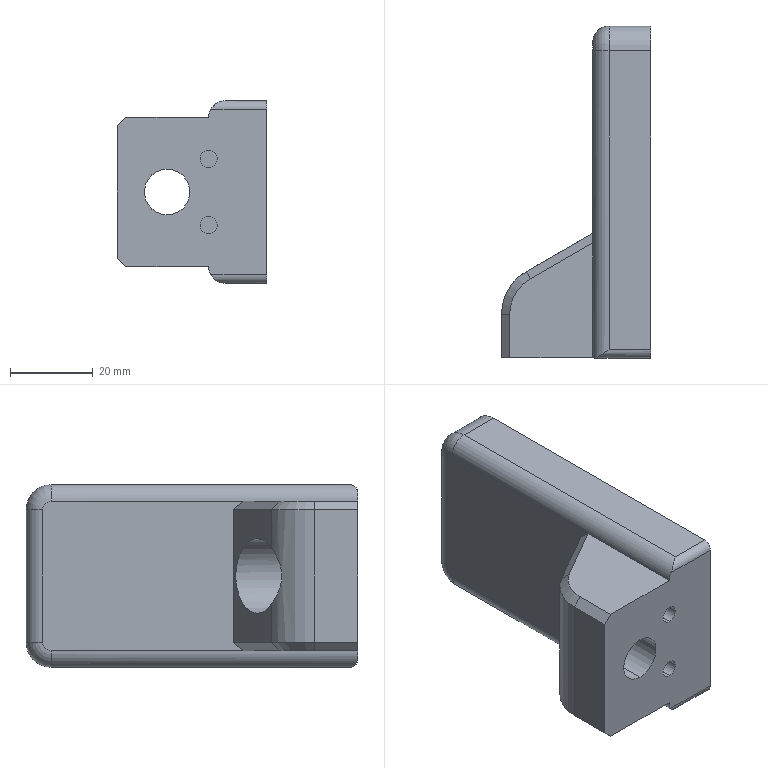Part | NX | features BREP 1 | 1 solid | 37 faces | box 36 x 80 x 44 mm | volume 61512 mm3 | plane 17 | cylinder 16 | cone 2 | torus 2 | commonest cylinder face diameters 4.1 x4 8 x3 4 x2 11 x2 12 x2 18 x2
STEP:
#1=CARTESIAN_POINT('',(-84.,294.703,-10.05));
#2=VERTEX_POINT('',#1);
#3=CARTESIAN_POINT('',(-84.,294.703,-5.95));
#4=VERTEX_POINT('',#3);
#5=CARTESIAN_POINT('',(-84.,294.703,-8.));
#6=DIRECTION('',(0.,-1.,0.));
#7=DIRECTION('',(0.,0.,1.));
#8=AXIS2_PLACEMENT_3D('',#5,#6,#7);
#9=CIRCLE('',#8,2.05);
#10=EDGE_CURVE('',#2,#4,#9,.T.);
#11=ORIENTED_EDGE('',*,*,#10,.F.);
#12=CARTESIAN_POINT('',(-84.,284.703,-10.05));
#13=VERTEX_POINT('',#12);
#14=CARTESIAN_POINT('',(-84.,294.703,-10.05));
#15=DIRECTION('',(0.,-1.,0.));
#16=VECTOR('',#15,1000.);
#17=LINE('',#14,#16);
#18=EDGE_CURVE('',#2,#13,#17,.T.);
#19=ORIENTED_EDGE('',*,*,#18,.T.);
#20=CARTESIAN_POINT('',(-84.,284.703,-5.95));
#21=VERTEX_POINT('',#20);
#22=CARTESIAN_POINT('',(-84.,284.703,-8.));
#23=DIRECTION('',(0.,-1.,0.));
#24=DIRECTION('',(0.,0.,1.));
#25=AXIS2_PLACEMENT_3D('',#22,#23,#24);
#26=CIRCLE('',#25,2.05);
#27=EDGE_CURVE('',#13,#21,#26,.T.);
#28=ORIENTED_EDGE('',*,*,#27,.T.);
#29=CARTESIAN_POINT('',(-84.,294.703,-5.95));
#30=DIRECTION('',(0.,1.,0.));
#31=VECTOR('',#30,1000.);
#32=LINE('',#29,#31);
#33=EDGE_CURVE('',#21,#4,#32,.T.);
#34=ORIENTED_EDGE('',*,*,#33,.T.);
#35=EDGE_LOOP('',(#11,#19,#28,#34));
#36=FACE_BOUND('',#35,.T.);
#37=CARTESIAN_POINT('',(-84.,294.703,-8.));
#38=DIRECTION('',(0.,-1.,0.));
#39=DIRECTION('',(0.,0.,-1.));
#40=AXIS2_PLACEMENT_3D('',#37,#38,#39);
#41=CYLINDRICAL_SURFACE('',#40,2.05);
#42=ADVANCED_FACE('',(#36),#41,.F.);
#43=CARTESIAN_POINT('',(-84.,294.703,5.95));
#44=VERTEX_POINT('',#43);
#45=CARTESIAN_POINT('',(-84.,294.703,10.05));
#46=VERTEX_POINT('',#45);
#47=CARTESIAN_POINT('',(-84.,294.703,8.));
#48=DIRECTION('',(0.,-1.,0.));
#49=DIRECTION('',(0.,0.,1.));
#50=AXIS2_PLACEMENT_3D('',#47,#48,#49);
#51=CIRCLE('',#50,2.05);
#52=EDGE_CURVE('',#44,#46,#51,.T.);
#53=ORIENTED_EDGE('',*,*,#52,.F.);
#54=CARTESIAN_POINT('',(-84.,284.703,5.95));
#55=VERTEX_POINT('',#54);
#56=CARTESIAN_POINT('',(-84.,294.703,5.95));
#57=DIRECTION('',(0.,1.,0.));
#58=VECTOR('',#57,1000.);
#59=LINE('',#56,#58);
#60=EDGE_CURVE('',#55,#44,#59,.T.);
#61=ORIENTED_EDGE('',*,*,#60,.F.);
#62=CARTESIAN_POINT('',(-84.,284.703,10.05));
#63=VERTEX_POINT('',#62);
#64=CARTESIAN_POINT('',(-84.,284.703,8.));
#65=DIRECTION('',(0.,-1.,0.));
#66=DIRECTION('',(0.,0.,1.));
#67=AXIS2_PLACEMENT_3D('',#64,#65,#66);
#68=CIRCLE('',#67,2.05);
#69=EDGE_CURVE('',#55,#63,#68,.T.);
#70=ORIENTED_EDGE('',*,*,#69,.T.);
#71=CARTESIAN_POINT('',(-84.,294.703,10.05));
#72=DIRECTION('',(0.,-1.,0.));
#73=VECTOR('',#72,1000.);
#74=LINE('',#71,#73);
#75=EDGE_CURVE('',#46,#63,#74,.T.);
#76=ORIENTED_EDGE('',*,*,#75,.F.);
#77=EDGE_LOOP('',(#53,#61,#70,#76));
#78=FACE_BOUND('',#77,.T.);
#79=CARTESIAN_POINT('',(-84.,294.703,8.));
#80=DIRECTION('',(0.,-1.,0.));
#81=DIRECTION('',(0.,0.,-1.));
#82=AXIS2_PLACEMENT_3D('',#79,#80,#81);
#83=CYLINDRICAL_SURFACE('',#82,2.05);
#84=ADVANCED_FACE('',(#78),#83,.F.);
#85=CARTESIAN_POINT('',(-94.,292.703,-9.));
#86=VERTEX_POINT('',#85);
#87=CARTESIAN_POINT('',(-94.,292.703,9.));
#88=VERTEX_POINT('',#87);
#89=CARTESIAN_POINT('',(-94.,292.703,0.));
#90=DIRECTION('',(0.,-1.,0.));
#91=DIRECTION('',(0.,0.,-1.));
#92=AXIS2_PLACEMENT_3D('',#89,#90,#91);
#93=CIRCLE('',#92,9.);
#94=EDGE_CURVE('',#86,#88,#93,.T.);
#95=ORIENTED_EDGE('',*,*,#94,.T.);
#96=CARTESIAN_POINT('',(-94.,308.93,9.));
#97=VERTEX_POINT('',#96);
#98=CARTESIAN_POINT('',(-94.,259.248,9.));
#99=DIRECTION('',(0.,-1.,0.));
#100=VECTOR('',#99,1000.);
#101=LINE('',#98,#100);
#102=EDGE_CURVE('',#97,#88,#101,.T.);
#103=ORIENTED_EDGE('',*,*,#102,.F.);
#104=CARTESIAN_POINT('',(-94.,308.93,-9.));
#105=VERTEX_POINT('',#104);
#106=CARTESIAN_POINT('',(-94.,308.93,-9.));
#107=CARTESIAN_POINT('',(-76.,319.322,-9.));
#108=CARTESIAN_POINT('',(-76.,319.322,9.));
#109=CARTESIAN_POINT('',(-94.,308.93,9.));
#110=(BOUNDED_CURVE()B_SPLINE_CURVE(3,(#106,#107,#108,#109),.UNSPECIFIED.,.F.,.F.)B_SPLINE_CURVE_WITH_KNOTS((4,4),(0.,1.),.PIECEWISE_BEZIER_KNOTS.)CURVE()GEOMETRIC_REPRESENTATION_ITEM()RATIONAL_B_SPLINE_CURVE((1.,0.3333,0.3333,1.))REPRESENTATION_ITEM(''));
#111=EDGE_CURVE('',#105,#97,#110,.T.);
#112=ORIENTED_EDGE('',*,*,#111,.F.);
#113=CARTESIAN_POINT('',(-94.,259.248,-9.));
#114=DIRECTION('',(0.,1.,0.));
#115=VECTOR('',#114,1000.);
#116=LINE('',#113,#115);
#117=EDGE_CURVE('',#86,#105,#116,.T.);
#118=ORIENTED_EDGE('',*,*,#117,.F.);
#119=EDGE_LOOP('',(#95,#103,#112,#118));
#120=FACE_BOUND('',#119,.T.);
#121=CARTESIAN_POINT('',(-94.,259.248,0.));
#122=DIRECTION('',(0.,1.,0.));
#123=DIRECTION('',(0.,0.,1.));
#124=AXIS2_PLACEMENT_3D('',#121,#122,#123);
#125=CYLINDRICAL_SURFACE('',#124,9.);
#126=ADVANCED_FACE('',(#120),#125,.F.);
#127=CARTESIAN_POINT('',(-94.,292.703,-5.5));
#128=VERTEX_POINT('',#127);
#129=CARTESIAN_POINT('',(-94.,292.703,5.5));
#130=VERTEX_POINT('',#129);
#131=CARTESIAN_POINT('',(-94.,292.703,0.));
#132=DIRECTION('',(0.,-1.,0.));
#133=DIRECTION('',(0.,0.,-1.));
#134=AXIS2_PLACEMENT_3D('',#131,#132,#133);
#135=CIRCLE('',#134,5.5);
#136=EDGE_CURVE('',#128,#130,#135,.T.);
#137=ORIENTED_EDGE('',*,*,#136,.F.);
#138=CARTESIAN_POINT('',(-94.,284.703,-5.5));
#139=VERTEX_POINT('',#138);
#140=CARTESIAN_POINT('',(-94.,314.703,-5.5));
#141=DIRECTION('',(0.,1.,0.));
#142=VECTOR('',#141,1000.);
#143=LINE('',#140,#142);
#144=EDGE_CURVE('',#139,#128,#143,.T.);
#145=ORIENTED_EDGE('',*,*,#144,.F.);
#146=CARTESIAN_POINT('',(-94.,284.703,5.5));
#147=VERTEX_POINT('',#146);
#148=CARTESIAN_POINT('',(-94.,284.703,0.));
#149=DIRECTION('',(0.,-1.,0.));
#150=DIRECTION('',(0.,0.,1.));
#151=AXIS2_PLACEMENT_3D('',#148,#149,#150);
#152=CIRCLE('',#151,5.5);
#153=EDGE_CURVE('',#139,#147,#152,.T.);
#154=ORIENTED_EDGE('',*,*,#153,.T.);
#155=CARTESIAN_POINT('',(-94.,314.703,5.5));
#156=DIRECTION('',(0.,-1.,0.));
#157=VECTOR('',#156,1000.);
#158=LINE('',#155,#157);
#159=EDGE_CURVE('',#130,#147,#158,.T.);
#160=ORIENTED_EDGE('',*,*,#159,.F.);
#161=EDGE_LOOP('',(#137,#145,#154,#160));
#162=FACE_BOUND('',#161,.T.);
#163=CARTESIAN_POINT('',(-94.,314.703,0.));
#164=DIRECTION('',(0.,-1.,0.));
#165=DIRECTION('',(0.,0.,-1.));
#166=AXIS2_PLACEMENT_3D('',#163,#164,#165);
#167=CYLINDRICAL_SURFACE('',#166,5.5);
#168=ADVANCED_FACE('',(#162),#167,.F.);
#169=ORIENTED_EDGE('',*,*,#144,.T.);
#170=CARTESIAN_POINT('',(-94.,292.703,0.));
#171=DIRECTION('',(0.,-1.,0.));
#172=DIRECTION('',(0.,0.,-1.));
#173=AXIS2_PLACEMENT_3D('',#170,#171,#172);
#174=CIRCLE('',#173,5.5);
#175=EDGE_CURVE('',#130,#128,#174,.T.);
#176=ORIENTED_EDGE('',*,*,#175,.F.);
#177=ORIENTED_EDGE('',*,*,#159,.T.);
#178=CARTESIAN_POINT('',(-94.,284.703,0.));
#179=DIRECTION('',(0.,-1.,0.));
#180=DIRECTION('',(0.,0.,1.));
#181=AXIS2_PLACEMENT_3D('',#178,#179,#180);
#182=CIRCLE('',#181,5.5);
#183=EDGE_CURVE('',#147,#139,#182,.T.);
#184=ORIENTED_EDGE('',*,*,#183,.T.);
#185=EDGE_LOOP('',(#169,#176,#177,#184));
#186=FACE_BOUND('',#185,.T.);
#187=CARTESIAN_POINT('',(-94.,314.703,0.));
#188=DIRECTION('',(0.,-1.,0.));
#189=DIRECTION('',(0.,0.,-1.));
#190=AXIS2_PLACEMENT_3D('',#187,#188,#189);
#191=CYLINDRICAL_SURFACE('',#190,5.5);
#192=ADVANCED_FACE('',(#186),#191,.F.);
#193=CARTESIAN_POINT('',(-70.,286.703,-22.));
#194=VERTEX_POINT('',#193);
#195=CARTESIAN_POINT('',(-80.,286.703,-22.));
#196=VERTEX_POINT('',#195);
#197=CARTESIAN_POINT('',(-84.,286.703,-22.));
#198=DIRECTION('',(-1.,0.,0.));
#199=VECTOR('',#198,1000.);
#200=LINE('',#197,#199);
#201=EDGE_CURVE('',#194,#196,#200,.T.);
#202=ORIENTED_EDGE('',*,*,#201,.T.);
#203=CARTESIAN_POINT('',(-80.,358.703,-22.));
#204=VERTEX_POINT('',#203);
#205=CARTESIAN_POINT('',(-80.,284.703,-22.));
#206=DIRECTION('',(0.,1.,0.));
#207=VECTOR('',#206,1000.);
#208=LINE('',#205,#207);
#209=EDGE_CURVE('',#196,#204,#208,.T.);
#210=ORIENTED_EDGE('',*,*,#209,.T.);
#211=CARTESIAN_POINT('',(-70.,358.703,-22.));
#212=VERTEX_POINT('',#211);
#213=CARTESIAN_POINT('',(-84.,358.703,-22.));
#214=DIRECTION('',(1.,0.,0.));
#215=VECTOR('',#214,1000.);
#216=LINE('',#213,#215);
#217=EDGE_CURVE('',#204,#212,#216,.T.);
#218=ORIENTED_EDGE('',*,*,#217,.T.);
#219=CARTESIAN_POINT('',(-70.,284.703,-22.));
#220=DIRECTION('',(0.,-1.,0.));
#221=VECTOR('',#220,1000.);
#222=LINE('',#219,#221);
#223=EDGE_CURVE('',#212,#194,#222,.T.);
#224=ORIENTED_EDGE('',*,*,#223,.T.);
#225=EDGE_LOOP('',(#202,#210,#218,#224));
#226=FACE_BOUND('',#225,.T.);
#227=CARTESIAN_POINT('',(-84.,284.703,-22.));
#228=DIRECTION('',(0.,0.,1.));
#229=DIRECTION('',(0.,-1.,0.));
#230=AXIS2_PLACEMENT_3D('',#227,#228,#229);
#231=PLANE('',#230);
#232=ADVANCED_FACE('',(#226),#231,.F.);
#233=CARTESIAN_POINT('',(-84.,284.703,-8.));
#234=DIRECTION('',(0.,-1.,0.));
#235=DIRECTION('',(0.,0.,1.));
#236=AXIS2_PLACEMENT_3D('',#233,#234,#235);
#237=CIRCLE('',#236,2.05);
#238=EDGE_CURVE('',#21,#13,#237,.T.);
#239=ORIENTED_EDGE('',*,*,#238,.F.);
#240=ORIENTED_EDGE('',*,*,#27,.F.);
#241=EDGE_LOOP('',(#239,#240));
#242=FACE_BOUND('',#241,.T.);
#243=CARTESIAN_POINT('',(-84.,284.703,8.));
#244=DIRECTION('',(0.,-1.,0.));
#245=DIRECTION('',(0.,0.,1.));
#246=AXIS2_PLACEMENT_3D('',#243,#244,#245);
#247=CIRCLE('',#246,2.05);
#248=EDGE_CURVE('',#63,#55,#247,.T.);
#249=ORIENTED_EDGE('',*,*,#248,.F.);
#250=ORIENTED_EDGE('',*,*,#69,.F.);
#251=EDGE_LOOP('',(#249,#250));
#252=FACE_BOUND('',#251,.T.);
#253=CARTESIAN_POINT('',(-104.,284.703,-18.));
#254=VERTEX_POINT('',#253);
#255=CARTESIAN_POINT('',(-84.,284.703,-18.));
#256=VERTEX_POINT('',#255);
#257=CARTESIAN_POINT('',(-104.,284.703,-18.));
#258=DIRECTION('',(1.,0.,0.));
#259=VECTOR('',#258,1000.);
#260=LINE('',#257,#259);
#261=EDGE_CURVE('',#254,#256,#260,.T.);
#262=ORIENTED_EDGE('',*,*,#261,.T.);
#263=CARTESIAN_POINT('',(-83.464,284.703,-20.));
#264=VERTEX_POINT('',#263);
#265=CARTESIAN_POINT('',(-80.,284.703,-18.));
#266=DIRECTION('',(0.,-1.,0.));
#267=DIRECTION('',(0.,0.,-1.));
#268=AXIS2_PLACEMENT_3D('',#265,#266,#267);
#269=CIRCLE('',#268,4.);
#270=EDGE_CURVE('',#256,#264,#269,.T.);
#271=ORIENTED_EDGE('',*,*,#270,.T.);
#272=CARTESIAN_POINT('',(-70.,284.703,-20.));
#273=VERTEX_POINT('',#272);
#274=CARTESIAN_POINT('',(-84.,284.703,-20.));
#275=DIRECTION('',(1.,0.,0.));
#276=VECTOR('',#275,1000.);
#277=LINE('',#274,#276);
#278=EDGE_CURVE('',#264,#273,#277,.T.);
#279=ORIENTED_EDGE('',*,*,#278,.T.);
#280=CARTESIAN_POINT('',(-70.,284.703,20.));
#281=VERTEX_POINT('',#280);
#282=CARTESIAN_POINT('',(-70.,284.703,-22.));
#283=DIRECTION('',(0.,0.,1.));
#284=VECTOR('',#283,1000.);
#285=LINE('',#282,#284);
#286=EDGE_CURVE('',#273,#281,#285,.T.);
#287=ORIENTED_EDGE('',*,*,#286,.T.);
#288=CARTESIAN_POINT('',(-83.464,284.703,20.));
#289=VERTEX_POINT('',#288);
#290=CARTESIAN_POINT('',(-84.,284.703,20.));
#291=DIRECTION('',(-1.,0.,0.));
#292=VECTOR('',#291,1000.);
#293=LINE('',#290,#292);
#294=EDGE_CURVE('',#281,#289,#293,.T.);
#295=ORIENTED_EDGE('',*,*,#294,.T.);
#296=CARTESIAN_POINT('',(-84.,284.703,18.));
#297=VERTEX_POINT('',#296);
#298=CARTESIAN_POINT('',(-80.,284.703,18.));
#299=DIRECTION('',(0.,-1.,0.));
#300=DIRECTION('',(0.,0.,-1.));
#301=AXIS2_PLACEMENT_3D('',#298,#299,#300);
#302=CIRCLE('',#301,4.);
#303=EDGE_CURVE('',#289,#297,#302,.T.);
#304=ORIENTED_EDGE('',*,*,#303,.T.);
#305=CARTESIAN_POINT('',(-104.,284.703,18.));
#306=VERTEX_POINT('',#305);
#307=CARTESIAN_POINT('',(-76.,284.703,18.));
#308=DIRECTION('',(-1.,0.,0.));
#309=VECTOR('',#308,1000.);
#310=LINE('',#307,#309);
#311=EDGE_CURVE('',#297,#306,#310,.T.);
#312=ORIENTED_EDGE('',*,*,#311,.T.);
#313=CARTESIAN_POINT('',(-106.,284.703,16.));
#314=VERTEX_POINT('',#313);
#315=CARTESIAN_POINT('',(-104.,284.703,18.));
#316=DIRECTION('',(-0.7071,0.,-0.7071));
#317=VECTOR('',#316,1000.);
#318=LINE('',#315,#317);
#319=EDGE_CURVE('',#306,#314,#318,.T.);
#320=ORIENTED_EDGE('',*,*,#319,.T.);
#321=CARTESIAN_POINT('',(-106.,284.703,-16.));
#322=VERTEX_POINT('',#321);
#323=CARTESIAN_POINT('',(-106.,284.703,16.));
#324=DIRECTION('',(0.,0.,-1.));
#325=VECTOR('',#324,1000.);
#326=LINE('',#323,#325);
#327=EDGE_CURVE('',#314,#322,#326,.T.);
#328=ORIENTED_EDGE('',*,*,#327,.T.);
#329=CARTESIAN_POINT('',(-106.,284.703,-16.));
#330=DIRECTION('',(0.7071,0.,-0.7071));
#331=VECTOR('',#330,1000.);
#332=LINE('',#329,#331);
#333=EDGE_CURVE('',#322,#254,#332,.T.);
#334=ORIENTED_EDGE('',*,*,#333,.T.);
#335=EDGE_LOOP('',(#262,#271,#279,#287,#295,#304,#312,#320,#328,#334));
#336=FACE_BOUND('',#335,.T.);
#337=ORIENTED_EDGE('',*,*,#183,.F.);
#338=ORIENTED_EDGE('',*,*,#153,.F.);
#339=EDGE_LOOP('',(#337,#338));
#340=FACE_BOUND('',#339,.T.);
#341=CARTESIAN_POINT('',(-84.,284.703,-22.));
#342=DIRECTION('',(0.,1.,0.));
#343=DIRECTION('',(0.,0.,1.));
#344=AXIS2_PLACEMENT_3D('',#341,#342,#343);
#345=PLANE('',#344);
#346=ADVANCED_FACE('',(#242,#252,#336,#340),#345,.F.);
#347=CARTESIAN_POINT('',(-70.,358.703,22.));
#348=VERTEX_POINT('',#347);
#349=CARTESIAN_POINT('',(-80.,358.703,22.));
#350=VERTEX_POINT('',#349);
#351=CARTESIAN_POINT('',(-84.,358.703,22.));
#352=DIRECTION('',(-1.,0.,0.));
#353=VECTOR('',#352,1000.);
#354=LINE('',#351,#353);
#355=EDGE_CURVE('',#348,#350,#354,.T.);
#356=ORIENTED_EDGE('',*,*,#355,.T.);
#357=CARTESIAN_POINT('',(-80.,286.703,22.));
#358=VERTEX_POINT('',#357);
#359=CARTESIAN_POINT('',(-80.,284.703,22.));
#360=DIRECTION('',(0.,-1.,0.));
#361=VECTOR('',#360,1000.);
#362=LINE('',#359,#361);
#363=EDGE_CURVE('',#350,#358,#362,.T.);
#364=ORIENTED_EDGE('',*,*,#363,.T.);
#365=CARTESIAN_POINT('',(-70.,286.703,22.));
#366=VERTEX_POINT('',#365);
#367=CARTESIAN_POINT('',(-84.,286.703,22.));
#368=DIRECTION('',(1.,0.,0.));
#369=VECTOR('',#368,1000.);
#370=LINE('',#367,#369);
#371=EDGE_CURVE('',#358,#366,#370,.T.);
#372=ORIENTED_EDGE('',*,*,#371,.T.);
#373=CARTESIAN_POINT('',(-70.,284.703,22.));
#374=DIRECTION('',(0.,1.,0.));
#375=VECTOR('',#374,1000.);
#376=LINE('',#373,#375);
#377=EDGE_CURVE('',#366,#348,#376,.T.);
#378=ORIENTED_EDGE('',*,*,#377,.T.);
#379=EDGE_LOOP('',(#356,#364,#372,#378));
#380=FACE_BOUND('',#379,.T.);
#381=CARTESIAN_POINT('',(-84.,284.703,22.));
#382=DIRECTION('',(0.,0.,-1.));
#383=DIRECTION('',(0.,1.,0.));
#384=AXIS2_PLACEMENT_3D('',#381,#382,#383);
#385=PLANE('',#384);
#386=ADVANCED_FACE('',(#380),#385,.F.);
#387=CARTESIAN_POINT('',(-70.,364.703,-16.));
#388=VERTEX_POINT('',#387);
#389=CARTESIAN_POINT('',(-80.,364.703,-16.));
#390=VERTEX_POINT('',#389);
#391=CARTESIAN_POINT('',(-84.,364.703,-16.));
#392=DIRECTION('',(-1.,0.,0.));
#393=VECTOR('',#392,1000.);
#394=LINE('',#391,#393);
#395=EDGE_CURVE('',#388,#390,#394,.T.);
#396=ORIENTED_EDGE('',*,*,#395,.T.);
#397=CARTESIAN_POINT('',(-80.,364.703,16.));
#398=VERTEX_POINT('',#397);
#399=CARTESIAN_POINT('',(-80.,364.703,-22.));
#400=DIRECTION('',(0.,0.,1.));
#401=VECTOR('',#400,1000.);
#402=LINE('',#399,#401);
#403=EDGE_CURVE('',#390,#398,#402,.T.);
#404=ORIENTED_EDGE('',*,*,#403,.T.);
#405=CARTESIAN_POINT('',(-70.,364.703,16.));
#406=VERTEX_POINT('',#405);
#407=CARTESIAN_POINT('',(-84.,364.703,16.));
#408=DIRECTION('',(1.,0.,0.));
#409=VECTOR('',#408,1000.);
#410=LINE('',#407,#409);
#411=EDGE_CURVE('',#398,#406,#410,.T.);
#412=ORIENTED_EDGE('',*,*,#411,.T.);
#413=CARTESIAN_POINT('',(-70.,364.703,-22.));
#414=DIRECTION('',(0.,0.,-1.));
#415=VECTOR('',#414,1000.);
#416=LINE('',#413,#415);
#417=EDGE_CURVE('',#406,#388,#416,.T.);
#418=ORIENTED_EDGE('',*,*,#417,.T.);
#419=EDGE_LOOP('',(#396,#404,#412,#418));
#420=FACE_BOUND('',#419,.T.);
#421=CARTESIAN_POINT('',(-84.,364.703,-22.));
#422=DIRECTION('',(0.,-1.,0.));
#423=DIRECTION('',(0.,0.,-1.));
#424=AXIS2_PLACEMENT_3D('',#421,#422,#423);
#425=PLANE('',#424);
#426=ADVANCED_FACE('',(#420),#425,.F.);
#427=CARTESIAN_POINT('',(-84.,360.703,-16.));
#428=VERTEX_POINT('',#427);
#429=CARTESIAN_POINT('',(-84.,358.703,-18.));
#430=VERTEX_POINT('',#429);
#431=CARTESIAN_POINT('',(-84.,358.703,-16.));
#432=DIRECTION('',(-1.,0.,0.));
#433=DIRECTION('',(0.,1.,0.));
#434=AXIS2_PLACEMENT_3D('',#431,#432,#433);
#435=CIRCLE('',#434,2.);
#436=EDGE_CURVE('',#428,#430,#435,.T.);
#437=ORIENTED_EDGE('',*,*,#436,.T.);
#438=CARTESIAN_POINT('',(-84.,312.394,-18.));
#439=VERTEX_POINT('',#438);
#440=CARTESIAN_POINT('',(-84.,284.703,-18.));
#441=DIRECTION('',(0.,-1.,0.));
#442=VECTOR('',#441,1000.);
#443=LINE('',#440,#442);
#444=EDGE_CURVE('',#430,#439,#443,.T.);
#445=ORIENTED_EDGE('',*,*,#444,.T.);
#446=CARTESIAN_POINT('',(-84.,314.703,-16.));
#447=VERTEX_POINT('',#446);
#448=CARTESIAN_POINT('',(-84.,294.591,-33.418));
#449=DIRECTION('',(0.,0.7559,0.6547));
#450=VECTOR('',#449,1000.);
#451=LINE('',#448,#450);
#452=EDGE_CURVE('',#439,#447,#451,.T.);
#453=ORIENTED_EDGE('',*,*,#452,.T.);
#454=CARTESIAN_POINT('',(-84.,314.703,16.));
#455=VERTEX_POINT('',#454);
#456=CARTESIAN_POINT('',(-84.,314.703,-22.));
#457=DIRECTION('',(0.,0.,-1.));
#458=VECTOR('',#457,1000.);
#459=LINE('',#456,#458);
#460=EDGE_CURVE('',#455,#447,#459,.T.);
#461=ORIENTED_EDGE('',*,*,#460,.F.);
#462=CARTESIAN_POINT('',(-84.,312.394,18.));
#463=VERTEX_POINT('',#462);
#464=CARTESIAN_POINT('',(-84.,316.366,14.56));
#465=DIRECTION('',(0.,-0.7559,0.6547));
#466=VECTOR('',#465,1000.);
#467=LINE('',#464,#466);
#468=EDGE_CURVE('',#455,#463,#467,.T.);
#469=ORIENTED_EDGE('',*,*,#468,.T.);
#470=CARTESIAN_POINT('',(-84.,358.703,18.));
#471=VERTEX_POINT('',#470);
#472=CARTESIAN_POINT('',(-84.,284.703,18.));
#473=DIRECTION('',(0.,1.,0.));
#474=VECTOR('',#473,1000.);
#475=LINE('',#472,#474);
#476=EDGE_CURVE('',#463,#471,#475,.T.);
#477=ORIENTED_EDGE('',*,*,#476,.T.);
#478=CARTESIAN_POINT('',(-84.,360.703,16.));
#479=VERTEX_POINT('',#478);
#480=CARTESIAN_POINT('',(-84.,358.703,16.));
#481=DIRECTION('',(-1.,0.,0.));
#482=DIRECTION('',(0.,1.,0.));
#483=AXIS2_PLACEMENT_3D('',#480,#481,#482);
#484=CIRCLE('',#483,2.);
#485=EDGE_CURVE('',#471,#479,#484,.T.);
#486=ORIENTED_EDGE('',*,*,#485,.T.);
#487=CARTESIAN_POINT('',(-84.,360.703,-22.));
#488=DIRECTION('',(0.,0.,-1.));
#489=VECTOR('',#488,1000.);
#490=LINE('',#487,#489);
#491=EDGE_CURVE('',#479,#428,#490,.T.);
#492=ORIENTED_EDGE('',*,*,#491,.T.);
#493=EDGE_LOOP('',(#437,#445,#453,#461,#469,#477,#486,#492));
#494=FACE_BOUND('',#493,.T.);
#495=CARTESIAN_POINT('',(-84.,284.703,-22.));
#496=DIRECTION('',(1.,0.,0.));
#497=DIRECTION('',(0.,-1.,0.));
#498=AXIS2_PLACEMENT_3D('',#495,#496,#497);
#499=PLANE('',#498);
#500=ADVANCED_FACE('',(#494),#499,.F.);
#501=ORIENTED_EDGE('',*,*,#223,.F.);
#502=CARTESIAN_POINT('',(-70.,358.703,-16.));
#503=DIRECTION('',(1.,0.,0.));
#504=DIRECTION('',(0.,1.,0.));
#505=AXIS2_PLACEMENT_3D('',#502,#503,#504);
#506=CIRCLE('',#505,6.);
#507=EDGE_CURVE('',#212,#388,#506,.T.);
#508=ORIENTED_EDGE('',*,*,#507,.T.);
#509=ORIENTED_EDGE('',*,*,#417,.F.);
#510=CARTESIAN_POINT('',(-70.,358.703,16.));
#511=DIRECTION('',(1.,0.,0.));
#512=DIRECTION('',(0.,1.,0.));
#513=AXIS2_PLACEMENT_3D('',#510,#511,#512);
#514=CIRCLE('',#513,6.);
#515=EDGE_CURVE('',#406,#348,#514,.T.);
#516=ORIENTED_EDGE('',*,*,#515,.T.);
#517=ORIENTED_EDGE('',*,*,#377,.F.);
#518=CARTESIAN_POINT('',(-70.,286.703,20.));
#519=DIRECTION('',(1.,0.,0.));
#520=DIRECTION('',(0.,1.,0.));
#521=AXIS2_PLACEMENT_3D('',#518,#519,#520);
#522=CIRCLE('',#521,2.);
#523=EDGE_CURVE('',#366,#281,#522,.T.);
#524=ORIENTED_EDGE('',*,*,#523,.T.);
#525=ORIENTED_EDGE('',*,*,#286,.F.);
#526=CARTESIAN_POINT('',(-70.,286.703,-20.));
#527=DIRECTION('',(1.,0.,0.));
#528=DIRECTION('',(0.,1.,0.));
#529=AXIS2_PLACEMENT_3D('',#526,#527,#528);
#530=CIRCLE('',#529,2.);
#531=EDGE_CURVE('',#273,#194,#530,.T.);
#532=ORIENTED_EDGE('',*,*,#531,.T.);
#533=EDGE_LOOP('',(#501,#508,#509,#516,#517,#524,#525,#532));
#534=FACE_BOUND('',#533,.T.);
#535=CARTESIAN_POINT('',(-70.,284.703,-22.));
#536=DIRECTION('',(1.,0.,0.));
#537=DIRECTION('',(0.,-1.,0.));
#538=AXIS2_PLACEMENT_3D('',#535,#536,#537);
#539=PLANE('',#538);
#540=ADVANCED_FACE('',(#534),#539,.T.);
#541=ORIENTED_EDGE('',*,*,#278,.F.);
#542=CARTESIAN_POINT('',(-83.464,284.703,-20.));
#543=CARTESIAN_POINT('',(-83.065,284.703,-20.691));
#544=CARTESIAN_POINT('',(-81.925,285.344,-21.707));
#545=CARTESIAN_POINT('',(-80.637,286.253,-22.));
#546=CARTESIAN_POINT('',(-80.,286.703,-22.));
#547=B_SPLINE_CURVE_WITH_KNOTS('',3,(#542,#543,#544,#545,#546),.UNSPECIFIED.,.F.,.F.,(4,1,4),(0.,0.002341,0.004683),.UNSPECIFIED.);
#548=EDGE_CURVE('',#264,#196,#547,.T.);
#549=ORIENTED_EDGE('',*,*,#548,.T.);
#550=ORIENTED_EDGE('',*,*,#201,.F.);
#551=ORIENTED_EDGE('',*,*,#531,.F.);
#552=EDGE_LOOP('',(#541,#549,#550,#551));
#553=FACE_BOUND('',#552,.T.);
#554=CARTESIAN_POINT('',(-84.,286.703,-20.));
#555=DIRECTION('',(1.,0.,0.));
#556=DIRECTION('',(0.,-1.,0.));
#557=AXIS2_PLACEMENT_3D('',#554,#555,#556);
#558=CYLINDRICAL_SURFACE('',#557,2.);
#559=ADVANCED_FACE('',(#553),#558,.T.);
#560=ORIENTED_EDGE('',*,*,#371,.F.);
#561=CARTESIAN_POINT('',(-80.,286.703,22.));
#562=CARTESIAN_POINT('',(-80.636,286.254,22.));
#563=CARTESIAN_POINT('',(-81.916,285.348,21.716));
#564=CARTESIAN_POINT('',(-83.071,284.703,20.681));
#565=CARTESIAN_POINT('',(-83.464,284.703,20.));
#566=B_SPLINE_CURVE_WITH_KNOTS('',3,(#561,#562,#563,#564,#565),.UNSPECIFIED.,.F.,.F.,(4,1,4),(-0.00001265,0.002323,0.004658),.UNSPECIFIED.);
#567=EDGE_CURVE('',#358,#289,#566,.T.);
#568=ORIENTED_EDGE('',*,*,#567,.T.);
#569=ORIENTED_EDGE('',*,*,#294,.F.);
#570=ORIENTED_EDGE('',*,*,#523,.F.);
#571=EDGE_LOOP('',(#560,#568,#569,#570));
#572=FACE_BOUND('',#571,.T.);
#573=CARTESIAN_POINT('',(-84.,286.703,20.));
#574=DIRECTION('',(1.,0.,0.));
#575=DIRECTION('',(0.,-1.,0.));
#576=AXIS2_PLACEMENT_3D('',#573,#574,#575);
#577=CYLINDRICAL_SURFACE('',#576,2.);
#578=ADVANCED_FACE('',(#572),#577,.T.);
#579=CARTESIAN_POINT('',(-104.,295.074,-18.));
#580=VERTEX_POINT('',#579);
#581=CARTESIAN_POINT('',(-104.,314.703,-18.));
#582=DIRECTION('',(0.,-1.,0.));
#583=VECTOR('',#582,1000.);
#584=LINE('',#581,#583);
#585=EDGE_CURVE('',#580,#254,#584,.T.);
#586=ORIENTED_EDGE('',*,*,#585,.F.);
#587=CARTESIAN_POINT('',(-99.,303.734,-18.));
#588=VERTEX_POINT('',#587);
#589=CARTESIAN_POINT('',(-94.,295.074,-18.));
#590=DIRECTION('',(0.,0.,-1.));
#591=DIRECTION('',(1.,0.,0.));
#592=AXIS2_PLACEMENT_3D('',#589,#590,#591);
#593=CIRCLE('',#592,10.);
#594=EDGE_CURVE('',#580,#588,#593,.T.);
#595=ORIENTED_EDGE('',*,*,#594,.T.);
#596=CARTESIAN_POINT('',(-83.,312.971,-18.));
#597=DIRECTION('',(0.866,0.5,0.));
#598=VECTOR('',#597,1000.);
#599=LINE('',#596,#598);
#600=EDGE_CURVE('',#588,#439,#599,.T.);
#601=ORIENTED_EDGE('',*,*,#600,.T.);
#602=CARTESIAN_POINT('',(-84.,284.703,-18.));
#603=DIRECTION('',(0.,1.,0.));
#604=VECTOR('',#603,1000.);
#605=LINE('',#602,#604);
#606=EDGE_CURVE('',#256,#439,#605,.T.);
#607=ORIENTED_EDGE('',*,*,#606,.F.);
#608=ORIENTED_EDGE('',*,*,#261,.F.);
#609=EDGE_LOOP('',(#586,#595,#601,#607,#608));
#610=FACE_BOUND('',#609,.T.);
#611=CARTESIAN_POINT('',(-104.,314.703,-18.));
#612=DIRECTION('',(0.,0.,-1.));
#613=DIRECTION('',(-1.,0.,0.));
#614=AXIS2_PLACEMENT_3D('',#611,#612,#613);
#615=PLANE('',#614);
#616=ADVANCED_FACE('',(#610),#615,.T.);
#617=CARTESIAN_POINT('',(-99.,303.734,18.));
#618=VERTEX_POINT('',#617);
#619=CARTESIAN_POINT('',(-99.,303.734,18.));
#620=DIRECTION('',(-0.866,-0.5,0.));
#621=VECTOR('',#620,1000.);
#622=LINE('',#619,#621);
#623=EDGE_CURVE('',#463,#618,#622,.T.);
#624=ORIENTED_EDGE('',*,*,#623,.T.);
#625=CARTESIAN_POINT('',(-104.,295.074,18.));
#626=VERTEX_POINT('',#625);
#627=CARTESIAN_POINT('',(-94.,295.074,18.));
#628=DIRECTION('',(0.,0.,1.));
#629=DIRECTION('',(-1.,0.,0.));
#630=AXIS2_PLACEMENT_3D('',#627,#628,#629);
#631=CIRCLE('',#630,10.);
#632=EDGE_CURVE('',#618,#626,#631,.T.);
#633=ORIENTED_EDGE('',*,*,#632,.T.);
#634=CARTESIAN_POINT('',(-104.,314.703,18.));
#635=DIRECTION('',(0.,-1.,0.));
#636=VECTOR('',#635,1000.);
#637=LINE('',#634,#636);
#638=EDGE_CURVE('',#626,#306,#637,.T.);
#639=ORIENTED_EDGE('',*,*,#638,.T.);
#640=ORIENTED_EDGE('',*,*,#311,.F.);
#641=CARTESIAN_POINT('',(-84.,284.703,18.));
#642=DIRECTION('',(0.,-1.,0.));
#643=VECTOR('',#642,1000.);
#644=LINE('',#641,#643);
#645=EDGE_CURVE('',#463,#297,#644,.T.);
#646=ORIENTED_EDGE('',*,*,#645,.F.);
#647=EDGE_LOOP('',(#624,#633,#639,#640,#646));
#648=FACE_BOUND('',#647,.T.);
#649=CARTESIAN_POINT('',(-76.,314.703,18.));
#650=DIRECTION('',(0.,0.,1.));
#651=DIRECTION('',(1.,0.,0.));
#652=AXIS2_PLACEMENT_3D('',#649,#650,#651);
#653=PLANE('',#652);
#654=ADVANCED_FACE('',(#648),#653,.T.);
#655=CARTESIAN_POINT('',(-106.,295.074,-16.));
#656=VERTEX_POINT('',#655);
#657=CARTESIAN_POINT('',(-106.,314.703,-16.));
#658=DIRECTION('',(0.,-1.,0.));
#659=VECTOR('',#658,1000.);
#660=LINE('',#657,#659);
#661=EDGE_CURVE('',#656,#322,#660,.T.);
#662=ORIENTED_EDGE('',*,*,#661,.F.);
#663=CARTESIAN_POINT('',(-99.,295.074,-23.));
#664=DIRECTION('',(0.7071,0.,-0.7071));
#665=VECTOR('',#664,1000.);
#666=LINE('',#663,#665);
#667=EDGE_CURVE('',#656,#580,#666,.T.);
#668=ORIENTED_EDGE('',*,*,#667,.T.);
#669=ORIENTED_EDGE('',*,*,#585,.T.);
#670=ORIENTED_EDGE('',*,*,#333,.F.);
#671=EDGE_LOOP('',(#662,#668,#669,#670));
#672=FACE_BOUND('',#671,.T.);
#673=CARTESIAN_POINT('',(-106.,314.703,-16.));
#674=DIRECTION('',(-0.7071,0.,-0.7071));
#675=DIRECTION('',(-0.7071,0.,0.7071));
#676=AXIS2_PLACEMENT_3D('',#673,#674,#675);
#677=PLANE('',#676);
#678=ADVANCED_FACE('',(#672),#677,.T.);
#679=CARTESIAN_POINT('',(-106.,295.074,16.));
#680=VERTEX_POINT('',#679);
#681=CARTESIAN_POINT('',(-106.,314.703,16.));
#682=DIRECTION('',(0.,-1.,0.));
#683=VECTOR('',#682,1000.);
#684=LINE('',#681,#683);
#685=EDGE_CURVE('',#680,#314,#684,.T.);
#686=ORIENTED_EDGE('',*,*,#685,.F.);
#687=CARTESIAN_POINT('',(-106.,295.074,-16.));
#688=DIRECTION('',(0.,0.,-1.));
#689=VECTOR('',#688,1000.);
#690=LINE('',#687,#689);
#691=EDGE_CURVE('',#680,#656,#690,.T.);
#692=ORIENTED_EDGE('',*,*,#691,.T.);
#693=ORIENTED_EDGE('',*,*,#661,.T.);
#694=ORIENTED_EDGE('',*,*,#327,.F.);
#695=EDGE_LOOP('',(#686,#692,#693,#694));
#696=FACE_BOUND('',#695,.T.);
#697=CARTESIAN_POINT('',(-106.,314.703,16.));
#698=DIRECTION('',(-1.,0.,0.));
#699=DIRECTION('',(0.,0.,1.));
#700=AXIS2_PLACEMENT_3D('',#697,#698,#699);
#701=PLANE('',#700);
#702=ADVANCED_FACE('',(#696),#701,.T.);
#703=ORIENTED_EDGE('',*,*,#638,.F.);
#704=CARTESIAN_POINT('',(-99.,295.074,23.));
#705=DIRECTION('',(-0.7071,0.,-0.7071));
#706=VECTOR('',#705,1000.);
#707=LINE('',#704,#706);
#708=EDGE_CURVE('',#626,#680,#707,.T.);
#709=ORIENTED_EDGE('',*,*,#708,.T.);
#710=ORIENTED_EDGE('',*,*,#685,.T.);
#711=ORIENTED_EDGE('',*,*,#319,.F.);
#712=EDGE_LOOP('',(#703,#709,#710,#711));
#713=FACE_BOUND('',#712,.T.);
#714=CARTESIAN_POINT('',(-104.,314.703,18.));
#715=DIRECTION('',(-0.7071,0.,0.7071));
#716=DIRECTION('',(0.7071,0.,0.7071));
#717=AXIS2_PLACEMENT_3D('',#714,#715,#716);
#718=PLANE('',#717);
#719=ADVANCED_FACE('',(#713),#718,.T.);
#720=CARTESIAN_POINT('',(-100.,305.466,-16.));
#721=VERTEX_POINT('',#720);
#722=CARTESIAN_POINT('',(-100.,305.466,-6.708));
#723=VERTEX_POINT('',#722);
#724=CARTESIAN_POINT('',(-100.,305.466,16.));
#725=DIRECTION('',(0.,0.,1.));
#726=VECTOR('',#725,1000.);
#727=LINE('',#724,#726);
#728=EDGE_CURVE('',#721,#723,#727,.T.);
#729=ORIENTED_EDGE('',*,*,#728,.T.);
#730=CARTESIAN_POINT('',(-100.,305.466,-6.708));
#731=CARTESIAN_POINT('',(-98.331,306.429,-8.201));
#732=CARTESIAN_POINT('',(-96.239,307.637,-9.));
#733=CARTESIAN_POINT('',(-94.,308.93,-9.));
#734=(BOUNDED_CURVE()B_SPLINE_CURVE(3,(#730,#731,#732,#733),.UNSPECIFIED.,.F.,.F.)B_SPLINE_CURVE_WITH_KNOTS((4,4),(0.,1.),.PIECEWISE_BEZIER_KNOTS.)CURVE()GEOMETRIC_REPRESENTATION_ITEM()RATIONAL_B_SPLINE_CURVE((1.,0.9561,0.9561,1.))REPRESENTATION_ITEM(''));
#735=EDGE_CURVE('',#723,#105,#734,.T.);
#736=ORIENTED_EDGE('',*,*,#735,.T.);
#737=ORIENTED_EDGE('',*,*,#111,.T.);
#738=CARTESIAN_POINT('',(-100.,305.466,6.708));
#739=VERTEX_POINT('',#738);
#740=CARTESIAN_POINT('',(-94.,308.93,9.));
#741=CARTESIAN_POINT('',(-96.239,307.637,9.));
#742=CARTESIAN_POINT('',(-98.331,306.429,8.201));
#743=CARTESIAN_POINT('',(-100.,305.466,6.708));
#744=(BOUNDED_CURVE()B_SPLINE_CURVE(3,(#740,#741,#742,#743),.UNSPECIFIED.,.F.,.F.)B_SPLINE_CURVE_WITH_KNOTS((4,4),(0.,1.),.PIECEWISE_BEZIER_KNOTS.)CURVE()GEOMETRIC_REPRESENTATION_ITEM()RATIONAL_B_SPLINE_CURVE((1.,0.9561,0.9561,1.))REPRESENTATION_ITEM(''));
#745=EDGE_CURVE('',#97,#739,#744,.T.);
#746=ORIENTED_EDGE('',*,*,#745,.T.);
#747=CARTESIAN_POINT('',(-100.,305.466,16.));
#748=VERTEX_POINT('',#747);
#749=CARTESIAN_POINT('',(-100.,305.466,16.));
#750=DIRECTION('',(0.,0.,1.));
#751=VECTOR('',#750,1000.);
#752=LINE('',#749,#751);
#753=EDGE_CURVE('',#739,#748,#752,.T.);
#754=ORIENTED_EDGE('',*,*,#753,.T.);
#755=CARTESIAN_POINT('',(-84.,314.703,16.));
#756=DIRECTION('',(0.866,0.5,0.));
#757=VECTOR('',#756,1000.);
#758=LINE('',#755,#757);
#759=EDGE_CURVE('',#748,#455,#758,.T.);
#760=ORIENTED_EDGE('',*,*,#759,.T.);
#761=ORIENTED_EDGE('',*,*,#460,.T.);
#762=CARTESIAN_POINT('',(-100.,305.466,-16.));
#763=DIRECTION('',(-0.866,-0.5,0.));
#764=VECTOR('',#763,1000.);
#765=LINE('',#762,#764);
#766=EDGE_CURVE('',#447,#721,#765,.T.);
#767=ORIENTED_EDGE('',*,*,#766,.T.);
#768=EDGE_LOOP('',(#729,#736,#737,#746,#754,#760,#761,#767));
#769=FACE_BOUND('',#768,.T.);
#770=CARTESIAN_POINT('',(-84.,314.703,-34.));
#771=DIRECTION('',(0.5,-0.866,0.));
#772=DIRECTION('',(-0.866,-0.5,0.));
#773=AXIS2_PLACEMENT_3D('',#770,#771,#772);
#774=PLANE('',#773);
#775=ADVANCED_FACE('',(#769),#774,.F.);
#776=CARTESIAN_POINT('',(-100.,305.466,-6.708));
#777=CARTESIAN_POINT('',(-100.921,304.934,-5.884));
#778=CARTESIAN_POINT('',(-102.376,303.756,-3.954));
#779=CARTESIAN_POINT('',(-103.311,302.639,-0.00655));
#780=CARTESIAN_POINT('',(-102.381,303.751,3.947));
#781=CARTESIAN_POINT('',(-100.921,304.934,5.884));
#782=CARTESIAN_POINT('',(-100.,305.466,6.708));
#783=B_SPLINE_CURVE_WITH_KNOTS('',3,(#776,#777,#778,#779,#780,#781,#782),.UNSPECIFIED.,.F.,.F.,(4,1,1,1,4),(0.,0.003984,0.007968,0.01195,0.01594),.UNSPECIFIED.);
#784=EDGE_CURVE('',#723,#739,#783,.T.);
#785=ORIENTED_EDGE('',*,*,#784,.F.);
#786=ORIENTED_EDGE('',*,*,#728,.F.);
#787=CARTESIAN_POINT('',(-94.,295.074,-16.));
#788=DIRECTION('',(0.,0.,1.));
#789=DIRECTION('',(1.,0.,0.));
#790=AXIS2_PLACEMENT_3D('',#787,#788,#789);
#791=CIRCLE('',#790,12.);
#792=EDGE_CURVE('',#721,#656,#791,.T.);
#793=ORIENTED_EDGE('',*,*,#792,.T.);
#794=ORIENTED_EDGE('',*,*,#691,.F.);
#795=CARTESIAN_POINT('',(-94.,295.074,16.));
#796=DIRECTION('',(0.,0.,-1.));
#797=DIRECTION('',(-1.,0.,0.));
#798=AXIS2_PLACEMENT_3D('',#795,#796,#797);
#799=CIRCLE('',#798,12.);
#800=EDGE_CURVE('',#680,#748,#799,.T.);
#801=ORIENTED_EDGE('',*,*,#800,.T.);
#802=ORIENTED_EDGE('',*,*,#753,.F.);
#803=EDGE_LOOP('',(#785,#786,#793,#794,#801,#802));
#804=FACE_BOUND('',#803,.T.);
#805=CARTESIAN_POINT('',(-94.,295.074,-34.));
#806=DIRECTION('',(0.,0.,-1.));
#807=DIRECTION('',(-1.,0.,0.));
#808=AXIS2_PLACEMENT_3D('',#805,#806,#807);
#809=CYLINDRICAL_SURFACE('',#808,12.);
#810=ADVANCED_FACE('',(#804),#809,.T.);
#811=ORIENTED_EDGE('',*,*,#452,.F.);
#812=ORIENTED_EDGE('',*,*,#600,.F.);
#813=CARTESIAN_POINT('',(-100.,305.466,-16.));
#814=DIRECTION('',(0.3536,-0.6124,-0.7071));
#815=VECTOR('',#814,1000.);
#816=LINE('',#813,#815);
#817=EDGE_CURVE('',#721,#588,#816,.T.);
#818=ORIENTED_EDGE('',*,*,#817,.F.);
#819=ORIENTED_EDGE('',*,*,#766,.F.);
#820=EDGE_LOOP('',(#811,#812,#818,#819));
#821=FACE_BOUND('',#820,.T.);
#822=CARTESIAN_POINT('',(-84.,314.703,-16.));
#823=DIRECTION('',(-0.3536,0.6124,-0.7071));
#824=DIRECTION('',(-0.866,-0.5,0.));
#825=AXIS2_PLACEMENT_3D('',#822,#823,#824);
#826=PLANE('',#825);
#827=ADVANCED_FACE('',(#821),#826,.T.);
#828=ORIENTED_EDGE('',*,*,#667,.F.);
#829=ORIENTED_EDGE('',*,*,#792,.F.);
#830=ORIENTED_EDGE('',*,*,#817,.T.);
#831=ORIENTED_EDGE('',*,*,#594,.F.);
#832=EDGE_LOOP('',(#828,#829,#830,#831));
#833=FACE_BOUND('',#832,.T.);
#834=CARTESIAN_POINT('',(-94.,295.074,-18.));
#835=DIRECTION('',(0.,0.,1.));
#836=DIRECTION('',(1.,0.,0.));
#837=AXIS2_PLACEMENT_3D('',#834,#835,#836);
#838=CONICAL_SURFACE('',#837,10.,0.7854);
#839=ADVANCED_FACE('',(#833),#838,.T.);
#840=ORIENTED_EDGE('',*,*,#468,.F.);
#841=ORIENTED_EDGE('',*,*,#759,.F.);
#842=CARTESIAN_POINT('',(-99.,303.734,18.));
#843=DIRECTION('',(-0.3536,0.6124,-0.7071));
#844=VECTOR('',#843,1000.);
#845=LINE('',#842,#844);
#846=EDGE_CURVE('',#618,#748,#845,.T.);
#847=ORIENTED_EDGE('',*,*,#846,.F.);
#848=ORIENTED_EDGE('',*,*,#623,.F.);
#849=EDGE_LOOP('',(#840,#841,#847,#848));
#850=FACE_BOUND('',#849,.T.);
#851=CARTESIAN_POINT('',(-84.,314.703,16.));
#852=DIRECTION('',(-0.3536,0.6124,0.7071));
#853=DIRECTION('',(0.866,0.5,0.));
#854=AXIS2_PLACEMENT_3D('',#851,#852,#853);
#855=PLANE('',#854);
#856=ADVANCED_FACE('',(#850),#855,.T.);
#857=ORIENTED_EDGE('',*,*,#846,.T.);
#858=ORIENTED_EDGE('',*,*,#800,.F.);
#859=ORIENTED_EDGE('',*,*,#708,.F.);
#860=ORIENTED_EDGE('',*,*,#632,.F.);
#861=EDGE_LOOP('',(#857,#858,#859,#860));
#862=FACE_BOUND('',#861,.T.);
#863=CARTESIAN_POINT('',(-94.,295.074,18.));
#864=DIRECTION('',(0.,0.,-1.));
#865=DIRECTION('',(-1.,0.,0.));
#866=AXIS2_PLACEMENT_3D('',#863,#864,#865);
#867=CONICAL_SURFACE('',#866,10.,0.7854);
#868=ADVANCED_FACE('',(#862),#867,.T.);
#869=ORIENTED_EDGE('',*,*,#217,.F.);
#870=CARTESIAN_POINT('',(-80.,358.703,-16.));
#871=DIRECTION('',(1.,0.,0.));
#872=DIRECTION('',(0.,1.,0.));
#873=AXIS2_PLACEMENT_3D('',#870,#871,#872);
#874=CIRCLE('',#873,6.);
#875=EDGE_CURVE('',#204,#390,#874,.T.);
#876=ORIENTED_EDGE('',*,*,#875,.T.);
#877=ORIENTED_EDGE('',*,*,#395,.F.);
#878=ORIENTED_EDGE('',*,*,#507,.F.);
#879=EDGE_LOOP('',(#869,#876,#877,#878));
#880=FACE_BOUND('',#879,.T.);
#881=CARTESIAN_POINT('',(-84.,358.703,-16.));
#882=DIRECTION('',(1.,0.,0.));
#883=DIRECTION('',(0.,-1.,0.));
#884=AXIS2_PLACEMENT_3D('',#881,#882,#883);
#885=CYLINDRICAL_SURFACE('',#884,6.);
#886=ADVANCED_FACE('',(#880),#885,.T.);
#887=ORIENTED_EDGE('',*,*,#411,.F.);
#888=CARTESIAN_POINT('',(-80.,358.703,16.));
#889=DIRECTION('',(1.,0.,0.));
#890=DIRECTION('',(0.,1.,0.));
#891=AXIS2_PLACEMENT_3D('',#888,#889,#890);
#892=CIRCLE('',#891,6.);
#893=EDGE_CURVE('',#398,#350,#892,.T.);
#894=ORIENTED_EDGE('',*,*,#893,.T.);
#895=ORIENTED_EDGE('',*,*,#355,.F.);
#896=ORIENTED_EDGE('',*,*,#515,.F.);
#897=EDGE_LOOP('',(#887,#894,#895,#896));
#898=FACE_BOUND('',#897,.T.);
#899=CARTESIAN_POINT('',(-84.,358.703,16.));
#900=DIRECTION('',(1.,0.,0.));
#901=DIRECTION('',(0.,-1.,0.));
#902=AXIS2_PLACEMENT_3D('',#899,#900,#901);
#903=CYLINDRICAL_SURFACE('',#902,6.);
#904=ADVANCED_FACE('',(#898),#903,.T.);
#905=ORIENTED_EDGE('',*,*,#567,.F.);
#906=ORIENTED_EDGE('',*,*,#363,.F.);
#907=CARTESIAN_POINT('',(-80.,358.703,18.));
#908=DIRECTION('',(0.,1.,0.));
#909=DIRECTION('',(0.,0.,-1.));
#910=AXIS2_PLACEMENT_3D('',#907,#908,#909);
#911=CIRCLE('',#910,4.);
#912=EDGE_CURVE('',#471,#350,#911,.T.);
#913=ORIENTED_EDGE('',*,*,#912,.F.);
#914=ORIENTED_EDGE('',*,*,#476,.F.);
#915=ORIENTED_EDGE('',*,*,#645,.T.);
#916=ORIENTED_EDGE('',*,*,#303,.F.);
#917=EDGE_LOOP('',(#905,#906,#913,#914,#915,#916));
#918=FACE_BOUND('',#917,.T.);
#919=CARTESIAN_POINT('',(-80.,284.703,18.));
#920=DIRECTION('',(0.,1.,0.));
#921=DIRECTION('',(0.,0.,1.));
#922=AXIS2_PLACEMENT_3D('',#919,#920,#921);
#923=CYLINDRICAL_SURFACE('',#922,4.);
#924=ADVANCED_FACE('',(#918),#923,.T.);
#925=ORIENTED_EDGE('',*,*,#912,.T.);
#926=ORIENTED_EDGE('',*,*,#893,.F.);
#927=CARTESIAN_POINT('',(-80.,360.703,16.));
#928=DIRECTION('',(0.,0.,-1.));
#929=DIRECTION('',(0.,-1.,0.));
#930=AXIS2_PLACEMENT_3D('',#927,#928,#929);
#931=CIRCLE('',#930,4.);
#932=EDGE_CURVE('',#479,#398,#931,.T.);
#933=ORIENTED_EDGE('',*,*,#932,.F.);
#934=ORIENTED_EDGE('',*,*,#485,.F.);
#935=EDGE_LOOP('',(#925,#926,#933,#934));
#936=FACE_BOUND('',#935,.T.);
#937=CARTESIAN_POINT('',(-80.,358.703,16.));
#938=DIRECTION('',(1.,0.,0.));
#939=DIRECTION('',(0.,0.,-1.));
#940=AXIS2_PLACEMENT_3D('',#937,#938,#939);
#941=DEGENERATE_TOROIDAL_SURFACE('',#940,2.,4.,.T.);
#942=ADVANCED_FACE('',(#936),#941,.T.);
#943=ORIENTED_EDGE('',*,*,#932,.T.);
#944=ORIENTED_EDGE('',*,*,#403,.F.);
#945=CARTESIAN_POINT('',(-80.,360.703,-16.));
#946=DIRECTION('',(0.,0.,-1.));
#947=DIRECTION('',(0.,-1.,0.));
#948=AXIS2_PLACEMENT_3D('',#945,#946,#947);
#949=CIRCLE('',#948,4.);
#950=EDGE_CURVE('',#428,#390,#949,.T.);
#951=ORIENTED_EDGE('',*,*,#950,.F.);
#952=ORIENTED_EDGE('',*,*,#491,.F.);
#953=EDGE_LOOP('',(#943,#944,#951,#952));
#954=FACE_BOUND('',#953,.T.);
#955=CARTESIAN_POINT('',(-80.,360.703,-22.));
#956=DIRECTION('',(0.,0.,-1.));
#957=DIRECTION('',(0.,1.,0.));
#958=AXIS2_PLACEMENT_3D('',#955,#956,#957);
#959=CYLINDRICAL_SURFACE('',#958,4.);
#960=ADVANCED_FACE('',(#954),#959,.T.);
#961=ORIENTED_EDGE('',*,*,#950,.T.);
#962=ORIENTED_EDGE('',*,*,#875,.F.);
#963=CARTESIAN_POINT('',(-80.,358.703,-18.));
#964=DIRECTION('',(0.,-1.,0.));
#965=DIRECTION('',(0.,0.,1.));
#966=AXIS2_PLACEMENT_3D('',#963,#964,#965);
#967=CIRCLE('',#966,4.);
#968=EDGE_CURVE('',#430,#204,#967,.T.);
#969=ORIENTED_EDGE('',*,*,#968,.F.);
#970=ORIENTED_EDGE('',*,*,#436,.F.);
#971=EDGE_LOOP('',(#961,#962,#969,#970));
#972=FACE_BOUND('',#971,.T.);
#973=CARTESIAN_POINT('',(-80.,358.703,-16.));
#974=DIRECTION('',(1.,0.,0.));
#975=DIRECTION('',(0.,0.,-1.));
#976=AXIS2_PLACEMENT_3D('',#973,#974,#975);
#977=DEGENERATE_TOROIDAL_SURFACE('',#976,2.,4.,.T.);
#978=ADVANCED_FACE('',(#972),#977,.T.);
#979=ORIENTED_EDGE('',*,*,#968,.T.);
#980=ORIENTED_EDGE('',*,*,#209,.F.);
#981=ORIENTED_EDGE('',*,*,#548,.F.);
#982=ORIENTED_EDGE('',*,*,#270,.F.);
#983=ORIENTED_EDGE('',*,*,#606,.T.);
#984=ORIENTED_EDGE('',*,*,#444,.F.);
#985=EDGE_LOOP('',(#979,#980,#981,#982,#983,#984));
#986=FACE_BOUND('',#985,.T.);
#987=CARTESIAN_POINT('',(-80.,284.703,-18.));
#988=DIRECTION('',(0.,-1.,0.));
#989=DIRECTION('',(0.,0.,-1.));
#990=AXIS2_PLACEMENT_3D('',#987,#988,#989);
#991=CYLINDRICAL_SURFACE('',#990,4.);
#992=ADVANCED_FACE('',(#986),#991,.T.);
#993=ORIENTED_EDGE('',*,*,#94,.F.);
#994=CARTESIAN_POINT('',(-94.,292.703,0.));
#995=DIRECTION('',(0.,-1.,0.));
#996=DIRECTION('',(0.,0.,-1.));
#997=AXIS2_PLACEMENT_3D('',#994,#995,#996);
#998=CIRCLE('',#997,9.);
#999=EDGE_CURVE('',#88,#86,#998,.T.);
#1000=ORIENTED_EDGE('',*,*,#999,.F.);
#1001=EDGE_LOOP('',(#993,#1000));
#1002=FACE_BOUND('',#1001,.T.);
#1003=ORIENTED_EDGE('',*,*,#175,.T.);
#1004=ORIENTED_EDGE('',*,*,#136,.T.);
#1005=EDGE_LOOP('',(#1003,#1004));
#1006=FACE_BOUND('',#1005,.T.);
#1007=CARTESIAN_POINT('',(-84.,292.703,-22.));
#1008=DIRECTION('',(0.,1.,0.));
#1009=DIRECTION('',(0.,0.,1.));
#1010=AXIS2_PLACEMENT_3D('',#1007,#1008,#1009);
#1011=PLANE('',#1010);
#1012=ADVANCED_FACE('',(#1002,#1006),#1011,.T.);
#1013=ORIENTED_EDGE('',*,*,#102,.T.);
#1014=ORIENTED_EDGE('',*,*,#999,.T.);
#1015=ORIENTED_EDGE('',*,*,#117,.T.);
#1016=ORIENTED_EDGE('',*,*,#735,.F.);
#1017=ORIENTED_EDGE('',*,*,#784,.T.);
#1018=ORIENTED_EDGE('',*,*,#745,.F.);
#1019=EDGE_LOOP('',(#1013,#1014,#1015,#1016,#1017,#1018));
#1020=FACE_BOUND('',#1019,.T.);
#1021=CARTESIAN_POINT('',(-94.,259.248,0.));
#1022=DIRECTION('',(0.,1.,0.));
#1023=DIRECTION('',(0.,0.,1.));
#1024=AXIS2_PLACEMENT_3D('',#1021,#1022,#1023);
#1025=CYLINDRICAL_SURFACE('',#1024,9.);
#1026=ADVANCED_FACE('',(#1020),#1025,.F.);
#1027=ORIENTED_EDGE('',*,*,#60,.T.);
#1028=CARTESIAN_POINT('',(-84.,294.703,8.));
#1029=DIRECTION('',(0.,-1.,0.));
#1030=DIRECTION('',(0.,0.,1.));
#1031=AXIS2_PLACEMENT_3D('',#1028,#1029,#1030);
#1032=CIRCLE('',#1031,2.05);
#1033=EDGE_CURVE('',#46,#44,#1032,.T.);
#1034=ORIENTED_EDGE('',*,*,#1033,.F.);
#1035=ORIENTED_EDGE('',*,*,#75,.T.);
#1036=ORIENTED_EDGE('',*,*,#248,.T.);
#1037=EDGE_LOOP('',(#1027,#1034,#1035,#1036));
#1038=FACE_BOUND('',#1037,.T.);
#1039=CARTESIAN_POINT('',(-84.,294.703,8.));
#1040=DIRECTION('',(0.,-1.,0.));
#1041=DIRECTION('',(0.,0.,-1.));
#1042=AXIS2_PLACEMENT_3D('',#1039,#1040,#1041);
#1043=CYLINDRICAL_SURFACE('',#1042,2.05);
#1044=ADVANCED_FACE('',(#1038),#1043,.F.);
#1045=ORIENTED_EDGE('',*,*,#1033,.T.);
#1046=ORIENTED_EDGE('',*,*,#52,.T.);
#1047=EDGE_LOOP('',(#1045,#1046));
#1048=FACE_BOUND('',#1047,.T.);
#1049=CARTESIAN_POINT('',(-84.,294.703,8.));
#1050=DIRECTION('',(0.,-1.,0.));
#1051=DIRECTION('',(0.,0.,-1.));
#1052=AXIS2_PLACEMENT_3D('',#1049,#1050,#1051);
#1053=PLANE('',#1052);
#1054=ADVANCED_FACE('',(#1048),#1053,.T.);
#1055=ORIENTED_EDGE('',*,*,#18,.F.);
#1056=CARTESIAN_POINT('',(-84.,294.703,-8.));
#1057=DIRECTION('',(0.,-1.,0.));
#1058=DIRECTION('',(0.,0.,1.));
#1059=AXIS2_PLACEMENT_3D('',#1056,#1057,#1058);
#1060=CIRCLE('',#1059,2.05);
#1061=EDGE_CURVE('',#4,#2,#1060,.T.);
#1062=ORIENTED_EDGE('',*,*,#1061,.F.);
#1063=ORIENTED_EDGE('',*,*,#33,.F.);
#1064=ORIENTED_EDGE('',*,*,#238,.T.);
#1065=EDGE_LOOP('',(#1055,#1062,#1063,#1064));
#1066=FACE_BOUND('',#1065,.T.);
#1067=CARTESIAN_POINT('',(-84.,294.703,-8.));
#1068=DIRECTION('',(0.,-1.,0.));
#1069=DIRECTION('',(0.,0.,-1.));
#1070=AXIS2_PLACEMENT_3D('',#1067,#1068,#1069);
#1071=CYLINDRICAL_SURFACE('',#1070,2.05);
#1072=ADVANCED_FACE('',(#1066),#1071,.F.);
#1073=ORIENTED_EDGE('',*,*,#1061,.T.);
#1074=ORIENTED_EDGE('',*,*,#10,.T.);
#1075=EDGE_LOOP('',(#1073,#1074));
#1076=FACE_BOUND('',#1075,.T.);
#1077=CARTESIAN_POINT('',(-84.,294.703,-8.));
#1078=DIRECTION('',(0.,-1.,0.));
#1079=DIRECTION('',(0.,0.,-1.));
#1080=AXIS2_PLACEMENT_3D('',#1077,#1078,#1079);
#1081=PLANE('',#1080);
#1082=ADVANCED_FACE('',(#1076),#1081,.T.);
#1083=CLOSED_SHELL('',(#42,#84,#126,#168,#192,#232,#346,#386,#426,#500,#540,#559,#578,#616,#654,#678,#702,#719,#775,#810,#827,#839,#856,#868,#886,#904,#924,#942,#960,#978,#992,#1012,#1026,#1044,#1054,#1072,#1082));
#1084=MANIFOLD_SOLID_BREP('',#1083);
#1085=(LENGTH_UNIT()NAMED_UNIT(*)SI_UNIT(.MILLI.,.METRE.));
#1086=UNCERTAINTY_MEASURE_WITH_UNIT(LENGTH_MEASURE(0.0508),#1085,'','');
#1087=(NAMED_UNIT(*)PLANE_ANGLE_UNIT()SI_UNIT($,.RADIAN.));
#1088=(NAMED_UNIT(*)SI_UNIT($,.STERADIAN.)SOLID_ANGLE_UNIT());
#1089=(GEOMETRIC_REPRESENTATION_CONTEXT(3)GLOBAL_UNCERTAINTY_ASSIGNED_CONTEXT((#1086))GLOBAL_UNIT_ASSIGNED_CONTEXT((#1085,#1087,#1088))REPRESENTATION_CONTEXT('',''));
#1090=ADVANCED_BREP_SHAPE_REPRESENTATION('',(#1084),#1089);